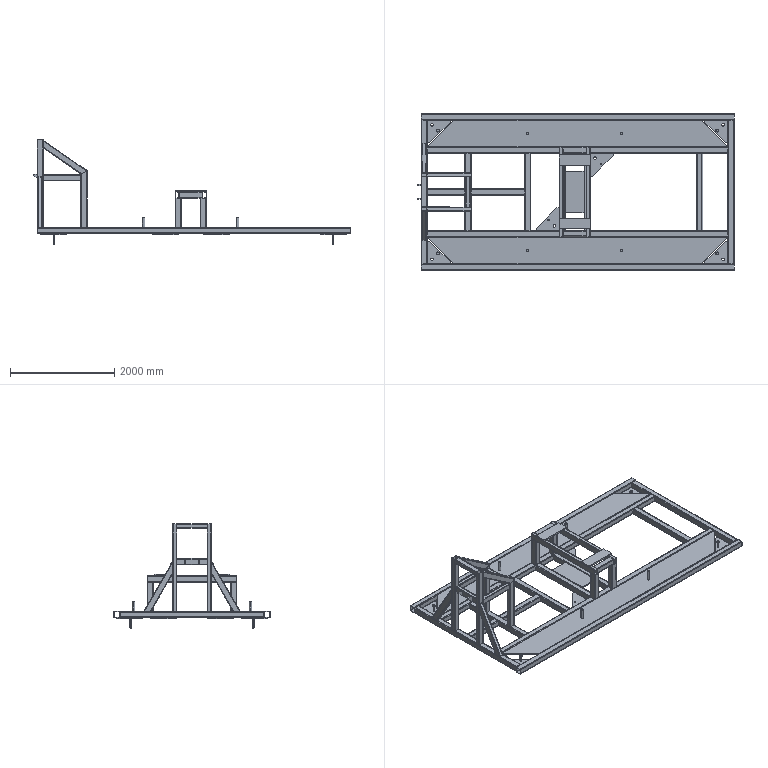Part | SolidWorks | features ReferencePattern 10, MirrorCompFeat 5, CompositeCurve 1 | 55 solids | 2074 faces | box 6060 x 3000 x 1995 mm | volume 369969133 mm3 | cylinder 1524 | plane 490 | cone 40 | spline 12 | torus 8 | commonest cylinder face diameters 30 x1212 32 x88 16 x76 12 x60 24 x60 50 x12